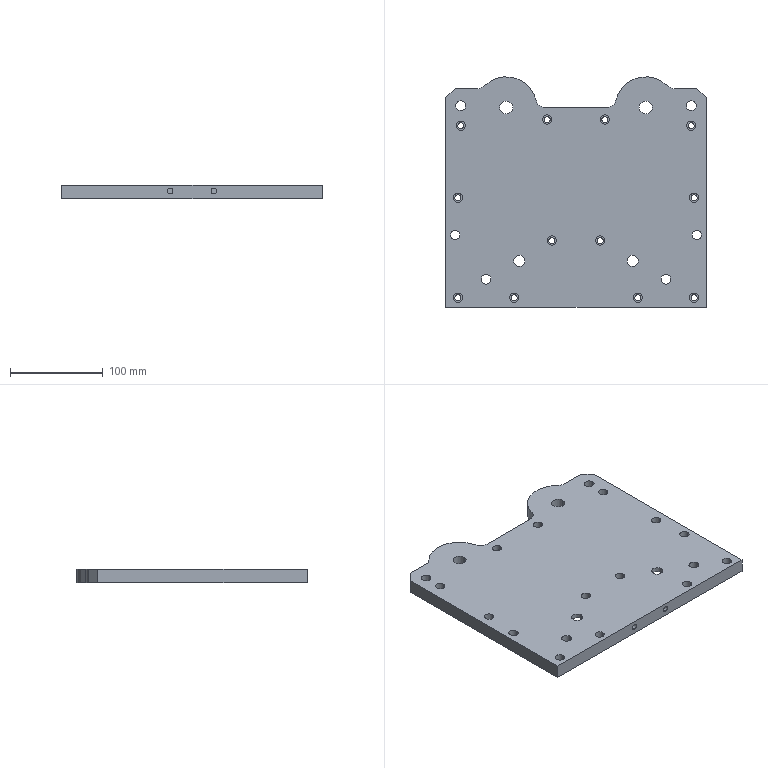Part | SolidWorks | features Cut 14, ICE 14, Fillet 2, Chamfer 1, Extrusion 1 | 1 solid | 148 faces | box 280 x 247.673 x 15 mm | volume 750844 mm3 | cylinder 103 | plane 45 | commonest cylinder face diameters 10 x28 6.5 x24 38 x11 10.5 x8 4 x6 6 x4